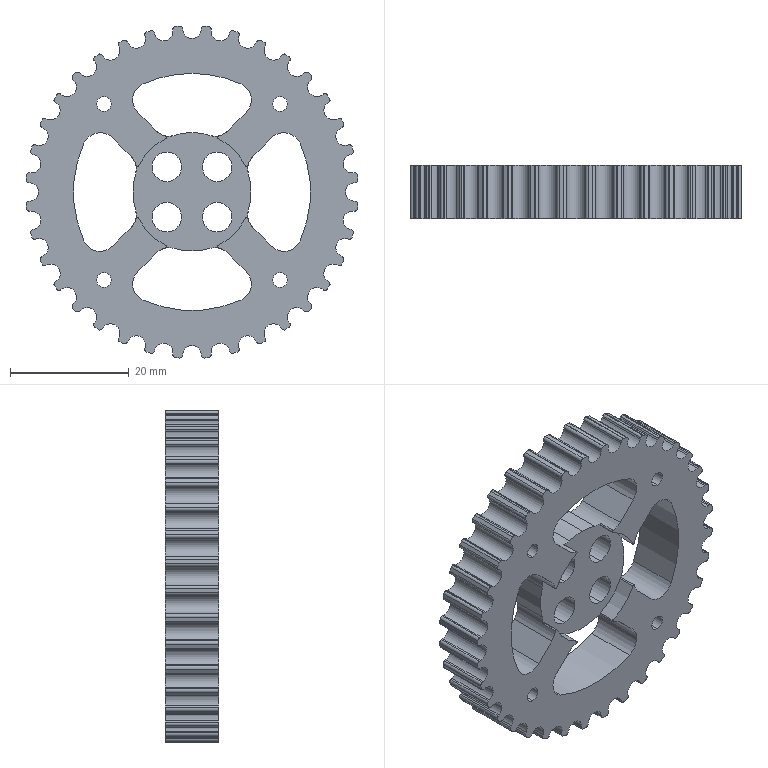Part | SolidWorks | features ICE 6, Chamfer 1, CirPattern 1, Fillet 1, Revolution 1 | 1 solid | 322 faces | box 56.006 x 9 x 56.006 mm | volume 12826 mm3 | cylinder 239 | plane 83 | commonest cylinder face diameters 0.96 x90 3.12 x53 56.16 x36 6 x20 0.4 x10 2.5 x8